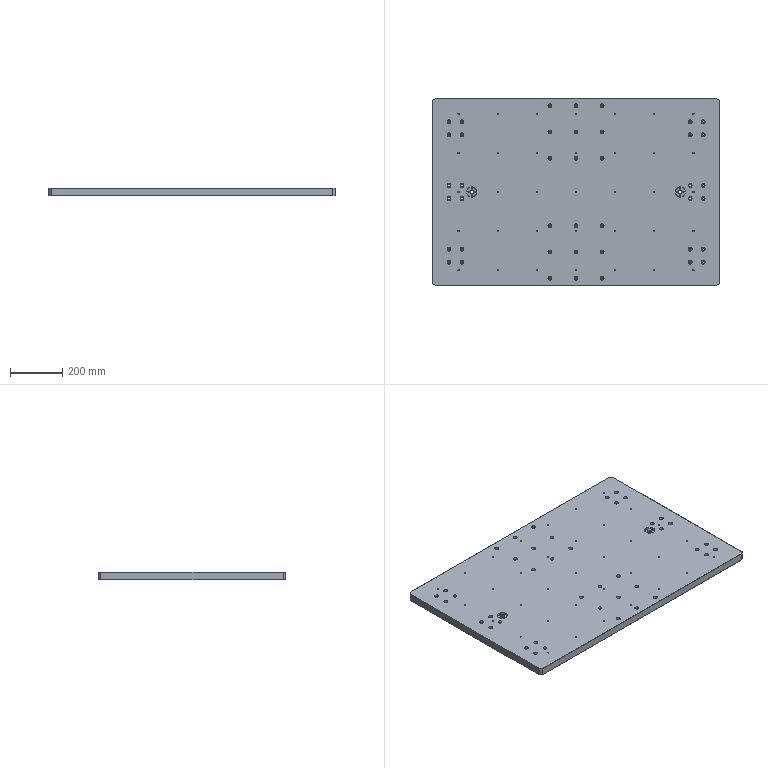Part | STEP file | TJ-DHQM-004-001 | 1 solid | 340 faces | box 1100 x 720 x 30 mm | volume 23583898 mm3 | cylinder 262 | plane 70 | cone 8 | commonest cylinder face diameters 9 x84 15 x84 5 x70 4.2 x16 12 x4 37 x4